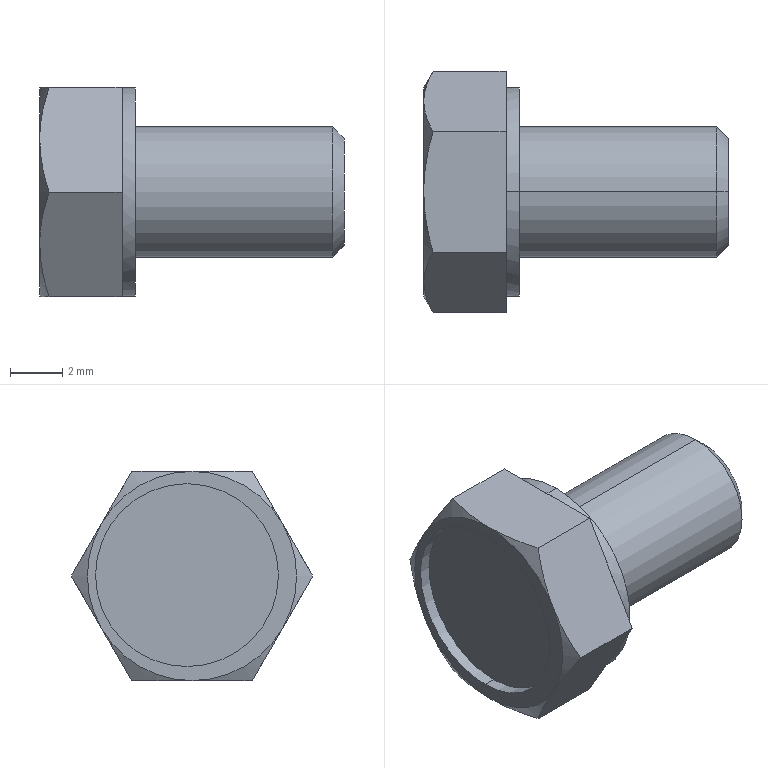Part | STEP file | formed hex screw_am_B18.2.3.2M - Formed hex screw, M5 x 0.8 x 8 --8WN | 1 solid | 30 faces | box 11.65 x 9.238 x 8 mm | volume 337.223 mm3 | plane 16 | cone 8 | cylinder 6 | commonest cylinder face diameters 5 x2 7 x2 8 x2